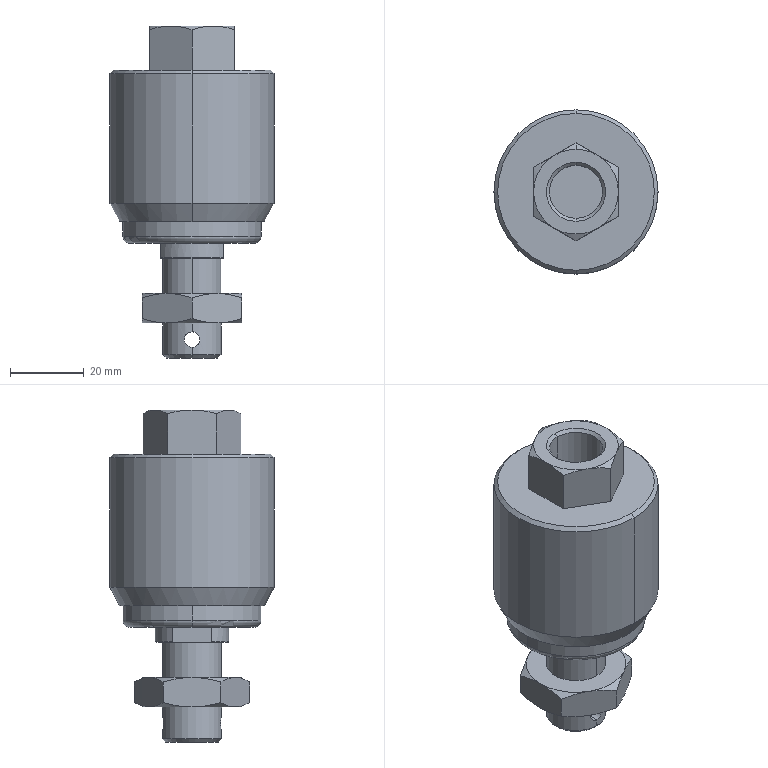Part | SolidWorks | features BaseBody 1 | 1 solid | 78 faces | box 44.5 x 44.5 x 90 mm | volume 80904 mm3 | cone 37 | plane 24 | cylinder 15 | torus 2 | commonest cylinder face diameters 16 x4 20 x3 4.2 x2 14.376 x2 37.5 x2 44.5 x2